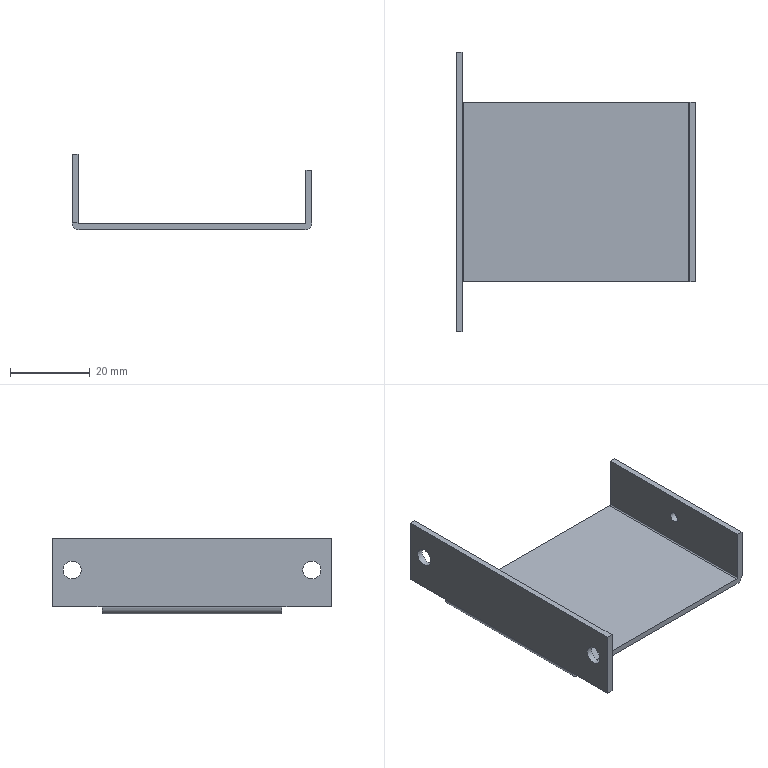Part | STEP file | FHD-021-008-02 limit block | 1 solid | 21 faces | box 60 x 70 x 19 mm | volume 6672 mm3 | plane 14 | cylinder 7 | commonest cylinder face diameters 0.6 x2 3.6 x2 4.5 x2 2.5 x1